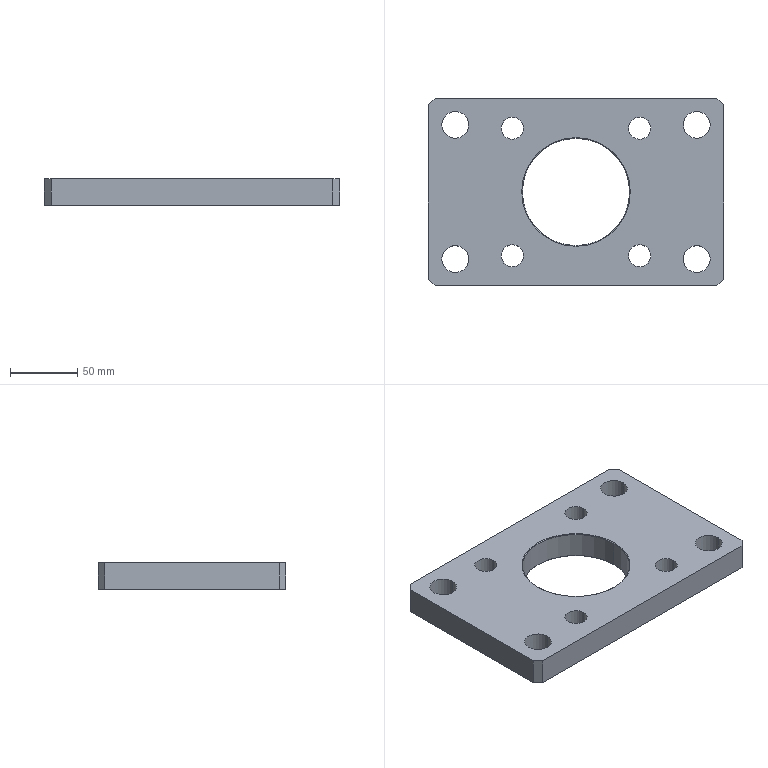Part | SolidWorks | features BaseBody 1 | 1 solid | 32 faces | box 220 x 140 x 20 mm | volume 472167 mm3 | cylinder 18 | plane 10 | cone 4 | commonest cylinder face diameters 16.5 x8 20 x8 80 x2
STEP:
#1=CARTESIAN_POINT('',(-40.,0.,19.5));
#2=VERTEX_POINT('',#1);
#3=CARTESIAN_POINT('',(40.,0.,19.5));
#4=VERTEX_POINT('',#3);
#5=CARTESIAN_POINT('',(0.,0.,19.5));
#6=DIRECTION('',(0.,0.,1.));
#7=DIRECTION('',(1.,0.,0.));
#8=AXIS2_PLACEMENT_3D('',#5,#6,#7);
#9=CIRCLE('',#8,40.);
#10=EDGE_CURVE('',#2,#4,#9,.T.);
#11=ORIENTED_EDGE('',*,*,#10,.F.);
#12=CARTESIAN_POINT('',(-40.5,0.,20.));
#13=VERTEX_POINT('',#12);
#14=CARTESIAN_POINT('',(-40.,0.,19.5));
#15=DIRECTION('',(-0.7071,0.,0.7071));
#16=VECTOR('',#15,1000.);
#17=LINE('',#14,#16);
#18=EDGE_CURVE('',#2,#13,#17,.T.);
#19=ORIENTED_EDGE('',*,*,#18,.T.);
#20=CARTESIAN_POINT('',(40.5,0.,20.));
#21=VERTEX_POINT('',#20);
#22=CARTESIAN_POINT('',(0.,0.,20.));
#23=DIRECTION('',(0.,0.,-1.));
#24=DIRECTION('',(1.,0.,0.));
#25=AXIS2_PLACEMENT_3D('',#22,#23,#24);
#26=CIRCLE('',#25,40.5);
#27=EDGE_CURVE('',#21,#13,#26,.T.);
#28=ORIENTED_EDGE('',*,*,#27,.F.);
#29=CARTESIAN_POINT('',(40.,0.,19.5));
#30=DIRECTION('',(0.7071,0.,0.7071));
#31=VECTOR('',#30,1000.);
#32=LINE('',#29,#31);
#33=EDGE_CURVE('',#4,#21,#32,.T.);
#34=ORIENTED_EDGE('',*,*,#33,.F.);
#35=EDGE_LOOP('',(#11,#19,#28,#34));
#36=FACE_OUTER_BOUND('',#35,.T.);
#37=CARTESIAN_POINT('',(0.,0.,19.5));
#38=DIRECTION('',(0.,0.,1.));
#39=DIRECTION('',(1.,0.,0.));
#40=AXIS2_PLACEMENT_3D('',#37,#38,#39);
#41=CONICAL_SURFACE('',#40,40.,0.7854);
#42=ADVANCED_FACE('',(#36),#41,.F.);
#43=CARTESIAN_POINT('',(40.,0.,0.5));
#44=VERTEX_POINT('',#43);
#45=CARTESIAN_POINT('',(-40.,0.,0.5));
#46=VERTEX_POINT('',#45);
#47=CARTESIAN_POINT('',(0.,0.,0.5));
#48=DIRECTION('',(0.,0.,-1.));
#49=DIRECTION('',(1.,0.,0.));
#50=AXIS2_PLACEMENT_3D('',#47,#48,#49);
#51=CIRCLE('',#50,40.);
#52=EDGE_CURVE('',#44,#46,#51,.T.);
#53=ORIENTED_EDGE('',*,*,#52,.F.);
#54=CARTESIAN_POINT('',(40.5,0.,0.));
#55=VERTEX_POINT('',#54);
#56=CARTESIAN_POINT('',(40.5,0.,0.));
#57=DIRECTION('',(0.7071,0.,-0.7071));
#58=VECTOR('',#57,1000.);
#59=LINE('',#56,#58);
#60=EDGE_CURVE('',#44,#55,#59,.T.);
#61=ORIENTED_EDGE('',*,*,#60,.T.);
#62=CARTESIAN_POINT('',(-40.5,0.,0.));
#63=VERTEX_POINT('',#62);
#64=CARTESIAN_POINT('',(0.,0.,0.));
#65=DIRECTION('',(0.,0.,1.));
#66=DIRECTION('',(1.,0.,0.));
#67=AXIS2_PLACEMENT_3D('',#64,#65,#66);
#68=CIRCLE('',#67,40.5);
#69=EDGE_CURVE('',#63,#55,#68,.T.);
#70=ORIENTED_EDGE('',*,*,#69,.F.);
#71=CARTESIAN_POINT('',(-40.5,0.,0.));
#72=DIRECTION('',(-0.7071,0.,-0.7071));
#73=VECTOR('',#72,1000.);
#74=LINE('',#71,#73);
#75=EDGE_CURVE('',#46,#63,#74,.T.);
#76=ORIENTED_EDGE('',*,*,#75,.F.);
#77=EDGE_LOOP('',(#53,#61,#70,#76));
#78=FACE_OUTER_BOUND('',#77,.T.);
#79=CARTESIAN_POINT('',(0.,0.,0.));
#80=DIRECTION('',(0.,0.,-1.));
#81=DIRECTION('',(-1.,0.,0.));
#82=AXIS2_PLACEMENT_3D('',#79,#80,#81);
#83=CONICAL_SURFACE('',#82,40.5,0.7854);
#84=ADVANCED_FACE('',(#78),#83,.F.);
#85=CARTESIAN_POINT('',(39.25,47.5,0.));
#86=VERTEX_POINT('',#85);
#87=CARTESIAN_POINT('',(55.75,47.5,0.));
#88=VERTEX_POINT('',#87);
#89=CARTESIAN_POINT('',(47.5,47.5,0.));
#90=DIRECTION('',(0.,0.,1.));
#91=DIRECTION('',(1.,0.,0.));
#92=AXIS2_PLACEMENT_3D('',#89,#90,#91);
#93=CIRCLE('',#92,8.25);
#94=EDGE_CURVE('',#86,#88,#93,.T.);
#95=ORIENTED_EDGE('',*,*,#94,.F.);
#96=CARTESIAN_POINT('',(39.25,47.5,20.));
#97=VERTEX_POINT('',#96);
#98=CARTESIAN_POINT('',(39.25,47.5,20.));
#99=DIRECTION('',(0.,0.,1.));
#100=VECTOR('',#99,1000.);
#101=LINE('',#98,#100);
#102=EDGE_CURVE('',#86,#97,#101,.T.);
#103=ORIENTED_EDGE('',*,*,#102,.T.);
#104=CARTESIAN_POINT('',(55.75,47.5,20.));
#105=VERTEX_POINT('',#104);
#106=CARTESIAN_POINT('',(47.5,47.5,20.));
#107=DIRECTION('',(0.,0.,1.));
#108=DIRECTION('',(1.,0.,0.));
#109=AXIS2_PLACEMENT_3D('',#106,#107,#108);
#110=CIRCLE('',#109,8.25);
#111=EDGE_CURVE('',#97,#105,#110,.T.);
#112=ORIENTED_EDGE('',*,*,#111,.T.);
#113=CARTESIAN_POINT('',(55.75,47.5,20.));
#114=DIRECTION('',(0.,0.,1.));
#115=VECTOR('',#114,1000.);
#116=LINE('',#113,#115);
#117=EDGE_CURVE('',#88,#105,#116,.T.);
#118=ORIENTED_EDGE('',*,*,#117,.F.);
#119=EDGE_LOOP('',(#95,#103,#112,#118));
#120=FACE_OUTER_BOUND('',#119,.T.);
#121=CARTESIAN_POINT('',(47.5,47.5,20.));
#122=DIRECTION('',(0.,0.,1.));
#123=DIRECTION('',(1.,0.,0.));
#124=AXIS2_PLACEMENT_3D('',#121,#122,#123);
#125=CYLINDRICAL_SURFACE('',#124,8.25);
#126=ADVANCED_FACE('',(#120),#125,.F.);
#127=CARTESIAN_POINT('',(39.25,-47.5,0.));
#128=VERTEX_POINT('',#127);
#129=CARTESIAN_POINT('',(55.75,-47.5,0.));
#130=VERTEX_POINT('',#129);
#131=CARTESIAN_POINT('',(47.5,-47.5,0.));
#132=DIRECTION('',(0.,0.,1.));
#133=DIRECTION('',(1.,0.,0.));
#134=AXIS2_PLACEMENT_3D('',#131,#132,#133);
#135=CIRCLE('',#134,8.25);
#136=EDGE_CURVE('',#128,#130,#135,.T.);
#137=ORIENTED_EDGE('',*,*,#136,.F.);
#138=CARTESIAN_POINT('',(39.25,-47.5,20.));
#139=VERTEX_POINT('',#138);
#140=CARTESIAN_POINT('',(39.25,-47.5,20.));
#141=DIRECTION('',(0.,0.,1.));
#142=VECTOR('',#141,1000.);
#143=LINE('',#140,#142);
#144=EDGE_CURVE('',#128,#139,#143,.T.);
#145=ORIENTED_EDGE('',*,*,#144,.T.);
#146=CARTESIAN_POINT('',(55.75,-47.5,20.));
#147=VERTEX_POINT('',#146);
#148=CARTESIAN_POINT('',(47.5,-47.5,20.));
#149=DIRECTION('',(0.,0.,1.));
#150=DIRECTION('',(1.,0.,0.));
#151=AXIS2_PLACEMENT_3D('',#148,#149,#150);
#152=CIRCLE('',#151,8.25);
#153=EDGE_CURVE('',#139,#147,#152,.T.);
#154=ORIENTED_EDGE('',*,*,#153,.T.);
#155=CARTESIAN_POINT('',(55.75,-47.5,20.));
#156=DIRECTION('',(0.,0.,1.));
#157=VECTOR('',#156,1000.);
#158=LINE('',#155,#157);
#159=EDGE_CURVE('',#130,#147,#158,.T.);
#160=ORIENTED_EDGE('',*,*,#159,.F.);
#161=EDGE_LOOP('',(#137,#145,#154,#160));
#162=FACE_OUTER_BOUND('',#161,.T.);
#163=CARTESIAN_POINT('',(47.5,-47.5,20.));
#164=DIRECTION('',(0.,0.,1.));
#165=DIRECTION('',(1.,0.,0.));
#166=AXIS2_PLACEMENT_3D('',#163,#164,#165);
#167=CYLINDRICAL_SURFACE('',#166,8.25);
#168=ADVANCED_FACE('',(#162),#167,.F.);
#169=CARTESIAN_POINT('',(-55.75,-47.5,0.));
#170=VERTEX_POINT('',#169);
#171=CARTESIAN_POINT('',(-39.25,-47.5,0.));
#172=VERTEX_POINT('',#171);
#173=CARTESIAN_POINT('',(-47.5,-47.5,0.));
#174=DIRECTION('',(0.,0.,1.));
#175=DIRECTION('',(1.,0.,0.));
#176=AXIS2_PLACEMENT_3D('',#173,#174,#175);
#177=CIRCLE('',#176,8.25);
#178=EDGE_CURVE('',#170,#172,#177,.T.);
#179=ORIENTED_EDGE('',*,*,#178,.F.);
#180=CARTESIAN_POINT('',(-55.75,-47.5,20.));
#181=VERTEX_POINT('',#180);
#182=CARTESIAN_POINT('',(-55.75,-47.5,20.));
#183=DIRECTION('',(0.,0.,1.));
#184=VECTOR('',#183,1000.);
#185=LINE('',#182,#184);
#186=EDGE_CURVE('',#170,#181,#185,.T.);
#187=ORIENTED_EDGE('',*,*,#186,.T.);
#188=CARTESIAN_POINT('',(-39.25,-47.5,20.));
#189=VERTEX_POINT('',#188);
#190=CARTESIAN_POINT('',(-47.5,-47.5,20.));
#191=DIRECTION('',(0.,0.,1.));
#192=DIRECTION('',(1.,0.,0.));
#193=AXIS2_PLACEMENT_3D('',#190,#191,#192);
#194=CIRCLE('',#193,8.25);
#195=EDGE_CURVE('',#181,#189,#194,.T.);
#196=ORIENTED_EDGE('',*,*,#195,.T.);
#197=CARTESIAN_POINT('',(-39.25,-47.5,20.));
#198=DIRECTION('',(0.,0.,1.));
#199=VECTOR('',#198,1000.);
#200=LINE('',#197,#199);
#201=EDGE_CURVE('',#172,#189,#200,.T.);
#202=ORIENTED_EDGE('',*,*,#201,.F.);
#203=EDGE_LOOP('',(#179,#187,#196,#202));
#204=FACE_OUTER_BOUND('',#203,.T.);
#205=CARTESIAN_POINT('',(-47.5,-47.5,20.));
#206=DIRECTION('',(0.,0.,1.));
#207=DIRECTION('',(1.,0.,0.));
#208=AXIS2_PLACEMENT_3D('',#205,#206,#207);
#209=CYLINDRICAL_SURFACE('',#208,8.25);
#210=ADVANCED_FACE('',(#204),#209,.F.);
#211=CARTESIAN_POINT('',(-55.75,47.5,0.));
#212=VERTEX_POINT('',#211);
#213=CARTESIAN_POINT('',(-39.25,47.5,0.));
#214=VERTEX_POINT('',#213);
#215=CARTESIAN_POINT('',(-47.5,47.5,0.));
#216=DIRECTION('',(0.,0.,1.));
#217=DIRECTION('',(1.,0.,0.));
#218=AXIS2_PLACEMENT_3D('',#215,#216,#217);
#219=CIRCLE('',#218,8.25);
#220=EDGE_CURVE('',#212,#214,#219,.T.);
#221=ORIENTED_EDGE('',*,*,#220,.F.);
#222=CARTESIAN_POINT('',(-55.75,47.5,20.));
#223=VERTEX_POINT('',#222);
#224=CARTESIAN_POINT('',(-55.75,47.5,20.));
#225=DIRECTION('',(0.,0.,1.));
#226=VECTOR('',#225,1000.);
#227=LINE('',#224,#226);
#228=EDGE_CURVE('',#212,#223,#227,.T.);
#229=ORIENTED_EDGE('',*,*,#228,.T.);
#230=CARTESIAN_POINT('',(-39.25,47.5,20.));
#231=VERTEX_POINT('',#230);
#232=CARTESIAN_POINT('',(-47.5,47.5,20.));
#233=DIRECTION('',(0.,0.,1.));
#234=DIRECTION('',(1.,0.,0.));
#235=AXIS2_PLACEMENT_3D('',#232,#233,#234);
#236=CIRCLE('',#235,8.25);
#237=EDGE_CURVE('',#223,#231,#236,.T.);
#238=ORIENTED_EDGE('',*,*,#237,.T.);
#239=CARTESIAN_POINT('',(-39.25,47.5,20.));
#240=DIRECTION('',(0.,0.,1.));
#241=VECTOR('',#240,1000.);
#242=LINE('',#239,#241);
#243=EDGE_CURVE('',#214,#231,#242,.T.);
#244=ORIENTED_EDGE('',*,*,#243,.F.);
#245=EDGE_LOOP('',(#221,#229,#238,#244));
#246=FACE_OUTER_BOUND('',#245,.T.);
#247=CARTESIAN_POINT('',(-47.5,47.5,20.));
#248=DIRECTION('',(0.,0.,1.));
#249=DIRECTION('',(1.,0.,0.));
#250=AXIS2_PLACEMENT_3D('',#247,#248,#249);
#251=CYLINDRICAL_SURFACE('',#250,8.25);
#252=ADVANCED_FACE('',(#246),#251,.F.);
#253=CARTESIAN_POINT('',(-100.,50.,0.));
#254=VERTEX_POINT('',#253);
#255=CARTESIAN_POINT('',(-80.,50.,0.));
#256=VERTEX_POINT('',#255);
#257=CARTESIAN_POINT('',(-90.,50.,0.));
#258=DIRECTION('',(0.,0.,1.));
#259=DIRECTION('',(1.,0.,0.));
#260=AXIS2_PLACEMENT_3D('',#257,#258,#259);
#261=CIRCLE('',#260,10.);
#262=EDGE_CURVE('',#254,#256,#261,.T.);
#263=ORIENTED_EDGE('',*,*,#262,.F.);
#264=CARTESIAN_POINT('',(-100.,50.,20.));
#265=VERTEX_POINT('',#264);
#266=CARTESIAN_POINT('',(-100.,50.,20.));
#267=DIRECTION('',(0.,0.,1.));
#268=VECTOR('',#267,1000.);
#269=LINE('',#266,#268);
#270=EDGE_CURVE('',#254,#265,#269,.T.);
#271=ORIENTED_EDGE('',*,*,#270,.T.);
#272=CARTESIAN_POINT('',(-80.,50.,20.));
#273=VERTEX_POINT('',#272);
#274=CARTESIAN_POINT('',(-90.,50.,20.));
#275=DIRECTION('',(0.,0.,1.));
#276=DIRECTION('',(1.,0.,0.));
#277=AXIS2_PLACEMENT_3D('',#274,#275,#276);
#278=CIRCLE('',#277,10.);
#279=EDGE_CURVE('',#265,#273,#278,.T.);
#280=ORIENTED_EDGE('',*,*,#279,.T.);
#281=CARTESIAN_POINT('',(-80.,50.,20.));
#282=DIRECTION('',(0.,0.,1.));
#283=VECTOR('',#282,1000.);
#284=LINE('',#281,#283);
#285=EDGE_CURVE('',#256,#273,#284,.T.);
#286=ORIENTED_EDGE('',*,*,#285,.F.);
#287=EDGE_LOOP('',(#263,#271,#280,#286));
#288=FACE_OUTER_BOUND('',#287,.T.);
#289=CARTESIAN_POINT('',(-90.,50.,20.));
#290=DIRECTION('',(0.,0.,1.));
#291=DIRECTION('',(1.,0.,0.));
#292=AXIS2_PLACEMENT_3D('',#289,#290,#291);
#293=CYLINDRICAL_SURFACE('',#292,10.);
#294=ADVANCED_FACE('',(#288),#293,.F.);
#295=CARTESIAN_POINT('',(-100.,-50.,0.));
#296=VERTEX_POINT('',#295);
#297=CARTESIAN_POINT('',(-80.,-50.,0.));
#298=VERTEX_POINT('',#297);
#299=CARTESIAN_POINT('',(-90.,-50.,0.));
#300=DIRECTION('',(0.,0.,1.));
#301=DIRECTION('',(1.,0.,0.));
#302=AXIS2_PLACEMENT_3D('',#299,#300,#301);
#303=CIRCLE('',#302,10.);
#304=EDGE_CURVE('',#296,#298,#303,.T.);
#305=ORIENTED_EDGE('',*,*,#304,.F.);
#306=CARTESIAN_POINT('',(-100.,-50.,20.));
#307=VERTEX_POINT('',#306);
#308=CARTESIAN_POINT('',(-100.,-50.,20.));
#309=DIRECTION('',(0.,0.,1.));
#310=VECTOR('',#309,1000.);
#311=LINE('',#308,#310);
#312=EDGE_CURVE('',#296,#307,#311,.T.);
#313=ORIENTED_EDGE('',*,*,#312,.T.);
#314=CARTESIAN_POINT('',(-80.,-50.,20.));
#315=VERTEX_POINT('',#314);
#316=CARTESIAN_POINT('',(-90.,-50.,20.));
#317=DIRECTION('',(0.,0.,1.));
#318=DIRECTION('',(1.,0.,0.));
#319=AXIS2_PLACEMENT_3D('',#316,#317,#318);
#320=CIRCLE('',#319,10.);
#321=EDGE_CURVE('',#307,#315,#320,.T.);
#322=ORIENTED_EDGE('',*,*,#321,.T.);
#323=CARTESIAN_POINT('',(-80.,-50.,20.));
#324=DIRECTION('',(0.,0.,1.));
#325=VECTOR('',#324,1000.);
#326=LINE('',#323,#325);
#327=EDGE_CURVE('',#298,#315,#326,.T.);
#328=ORIENTED_EDGE('',*,*,#327,.F.);
#329=EDGE_LOOP('',(#305,#313,#322,#328));
#330=FACE_OUTER_BOUND('',#329,.T.);
#331=CARTESIAN_POINT('',(-90.,-50.,20.));
#332=DIRECTION('',(0.,0.,1.));
#333=DIRECTION('',(1.,0.,0.));
#334=AXIS2_PLACEMENT_3D('',#331,#332,#333);
#335=CYLINDRICAL_SURFACE('',#334,10.);
#336=ADVANCED_FACE('',(#330),#335,.F.);
#337=CARTESIAN_POINT('',(80.,50.,0.));
#338=VERTEX_POINT('',#337);
#339=CARTESIAN_POINT('',(100.,50.,0.));
#340=VERTEX_POINT('',#339);
#341=CARTESIAN_POINT('',(90.,50.,0.));
#342=DIRECTION('',(0.,0.,1.));
#343=DIRECTION('',(1.,0.,0.));
#344=AXIS2_PLACEMENT_3D('',#341,#342,#343);
#345=CIRCLE('',#344,10.);
#346=EDGE_CURVE('',#338,#340,#345,.T.);
#347=ORIENTED_EDGE('',*,*,#346,.F.);
#348=CARTESIAN_POINT('',(80.,50.,20.));
#349=VERTEX_POINT('',#348);
#350=CARTESIAN_POINT('',(80.,50.,20.));
#351=DIRECTION('',(0.,0.,1.));
#352=VECTOR('',#351,1000.);
#353=LINE('',#350,#352);
#354=EDGE_CURVE('',#338,#349,#353,.T.);
#355=ORIENTED_EDGE('',*,*,#354,.T.);
#356=CARTESIAN_POINT('',(100.,50.,20.));
#357=VERTEX_POINT('',#356);
#358=CARTESIAN_POINT('',(90.,50.,20.));
#359=DIRECTION('',(0.,0.,1.));
#360=DIRECTION('',(1.,0.,0.));
#361=AXIS2_PLACEMENT_3D('',#358,#359,#360);
#362=CIRCLE('',#361,10.);
#363=EDGE_CURVE('',#349,#357,#362,.T.);
#364=ORIENTED_EDGE('',*,*,#363,.T.);
#365=CARTESIAN_POINT('',(100.,50.,20.));
#366=DIRECTION('',(0.,0.,1.));
#367=VECTOR('',#366,1000.);
#368=LINE('',#365,#367);
#369=EDGE_CURVE('',#340,#357,#368,.T.);
#370=ORIENTED_EDGE('',*,*,#369,.F.);
#371=EDGE_LOOP('',(#347,#355,#364,#370));
#372=FACE_OUTER_BOUND('',#371,.T.);
#373=CARTESIAN_POINT('',(90.,50.,20.));
#374=DIRECTION('',(0.,0.,1.));
#375=DIRECTION('',(1.,0.,0.));
#376=AXIS2_PLACEMENT_3D('',#373,#374,#375);
#377=CYLINDRICAL_SURFACE('',#376,10.);
#378=ADVANCED_FACE('',(#372),#377,.F.);
#379=CARTESIAN_POINT('',(80.,-50.,0.));
#380=VERTEX_POINT('',#379);
#381=CARTESIAN_POINT('',(100.,-50.,0.));
#382=VERTEX_POINT('',#381);
#383=CARTESIAN_POINT('',(90.,-50.,0.));
#384=DIRECTION('',(0.,0.,1.));
#385=DIRECTION('',(1.,0.,0.));
#386=AXIS2_PLACEMENT_3D('',#383,#384,#385);
#387=CIRCLE('',#386,10.);
#388=EDGE_CURVE('',#380,#382,#387,.T.);
#389=ORIENTED_EDGE('',*,*,#388,.F.);
#390=CARTESIAN_POINT('',(80.,-50.,20.));
#391=VERTEX_POINT('',#390);
#392=CARTESIAN_POINT('',(80.,-50.,20.));
#393=DIRECTION('',(0.,0.,1.));
#394=VECTOR('',#393,1000.);
#395=LINE('',#392,#394);
#396=EDGE_CURVE('',#380,#391,#395,.T.);
#397=ORIENTED_EDGE('',*,*,#396,.T.);
#398=CARTESIAN_POINT('',(100.,-50.,20.));
#399=VERTEX_POINT('',#398);
#400=CARTESIAN_POINT('',(90.,-50.,20.));
#401=DIRECTION('',(0.,0.,1.));
#402=DIRECTION('',(1.,0.,0.));
#403=AXIS2_PLACEMENT_3D('',#400,#401,#402);
#404=CIRCLE('',#403,10.);
#405=EDGE_CURVE('',#391,#399,#404,.T.);
#406=ORIENTED_EDGE('',*,*,#405,.T.);
#407=CARTESIAN_POINT('',(100.,-50.,20.));
#408=DIRECTION('',(0.,0.,1.));
#409=VECTOR('',#408,1000.);
#410=LINE('',#407,#409);
#411=EDGE_CURVE('',#382,#399,#410,.T.);
#412=ORIENTED_EDGE('',*,*,#411,.F.);
#413=EDGE_LOOP('',(#389,#397,#406,#412));
#414=FACE_OUTER_BOUND('',#413,.T.);
#415=CARTESIAN_POINT('',(90.,-50.,20.));
#416=DIRECTION('',(0.,0.,1.));
#417=DIRECTION('',(1.,0.,0.));
#418=AXIS2_PLACEMENT_3D('',#415,#416,#417);
#419=CYLINDRICAL_SURFACE('',#418,10.);
#420=ADVANCED_FACE('',(#414),#419,.F.);
#421=ORIENTED_EDGE('',*,*,#10,.T.);
#422=CARTESIAN_POINT('',(40.,0.,20.));
#423=DIRECTION('',(0.,0.,-1.));
#424=VECTOR('',#423,1000.);
#425=LINE('',#422,#424);
#426=EDGE_CURVE('',#4,#44,#425,.T.);
#427=ORIENTED_EDGE('',*,*,#426,.T.);
#428=ORIENTED_EDGE('',*,*,#52,.T.);
#429=CARTESIAN_POINT('',(-40.,0.,20.));
#430=DIRECTION('',(0.,0.,-1.));
#431=VECTOR('',#430,1000.);
#432=LINE('',#429,#431);
#433=EDGE_CURVE('',#2,#46,#432,.T.);
#434=ORIENTED_EDGE('',*,*,#433,.F.);
#435=EDGE_LOOP('',(#421,#427,#428,#434));
#436=FACE_OUTER_BOUND('',#435,.T.);
#437=CARTESIAN_POINT('',(0.,0.,20.));
#438=DIRECTION('',(0.,0.,-1.));
#439=DIRECTION('',(-1.,0.,0.));
#440=AXIS2_PLACEMENT_3D('',#437,#438,#439);
#441=CYLINDRICAL_SURFACE('',#440,40.);
#442=ADVANCED_FACE('',(#436),#441,.F.);
#443=CARTESIAN_POINT('',(110.,65.,20.));
#444=VERTEX_POINT('',#443);
#445=CARTESIAN_POINT('',(105.,70.,20.));
#446=VERTEX_POINT('',#445);
#447=CARTESIAN_POINT('',(87.5,87.5,20.));
#448=DIRECTION('',(-0.7071,0.7071,0.));
#449=VECTOR('',#448,1000.);
#450=LINE('',#447,#449);
#451=EDGE_CURVE('',#444,#446,#450,.T.);
#452=ORIENTED_EDGE('',*,*,#451,.F.);
#453=CARTESIAN_POINT('',(110.,65.,0.));
#454=VERTEX_POINT('',#453);
#455=CARTESIAN_POINT('',(110.,65.,20.));
#456=DIRECTION('',(0.,0.,1.));
#457=VECTOR('',#456,1000.);
#458=LINE('',#455,#457);
#459=EDGE_CURVE('',#454,#444,#458,.T.);
#460=ORIENTED_EDGE('',*,*,#459,.F.);
#461=CARTESIAN_POINT('',(105.,70.,0.));
#462=VERTEX_POINT('',#461);
#463=CARTESIAN_POINT('',(105.,70.,0.));
#464=DIRECTION('',(0.7071,-0.7071,0.));
#465=VECTOR('',#464,1000.);
#466=LINE('',#463,#465);
#467=EDGE_CURVE('',#462,#454,#466,.T.);
#468=ORIENTED_EDGE('',*,*,#467,.F.);
#469=CARTESIAN_POINT('',(105.,70.,20.));
#470=DIRECTION('',(0.,0.,-1.));
#471=VECTOR('',#470,1000.);
#472=LINE('',#469,#471);
#473=EDGE_CURVE('',#446,#462,#472,.T.);
#474=ORIENTED_EDGE('',*,*,#473,.F.);
#475=EDGE_LOOP('',(#452,#460,#468,#474));
#476=FACE_OUTER_BOUND('',#475,.T.);
#477=CARTESIAN_POINT('',(105.,70.,20.));
#478=DIRECTION('',(-0.7071,-0.7071,0.));
#479=DIRECTION('',(-0.7071,0.7071,0.));
#480=AXIS2_PLACEMENT_3D('',#477,#478,#479);
#481=PLANE('',#480);
#482=ADVANCED_FACE('',(#476),#481,.F.);
#483=CARTESIAN_POINT('',(105.,-70.,20.));
#484=VERTEX_POINT('',#483);
#485=CARTESIAN_POINT('',(110.,-65.,20.));
#486=VERTEX_POINT('',#485);
#487=CARTESIAN_POINT('',(87.5,-87.5,20.));
#488=DIRECTION('',(0.7071,0.7071,0.));
#489=VECTOR('',#488,1000.);
#490=LINE('',#487,#489);
#491=EDGE_CURVE('',#484,#486,#490,.T.);
#492=ORIENTED_EDGE('',*,*,#491,.F.);
#493=CARTESIAN_POINT('',(105.,-70.,0.));
#494=VERTEX_POINT('',#493);
#495=CARTESIAN_POINT('',(105.,-70.,20.));
#496=DIRECTION('',(0.,0.,1.));
#497=VECTOR('',#496,1000.);
#498=LINE('',#495,#497);
#499=EDGE_CURVE('',#494,#484,#498,.T.);
#500=ORIENTED_EDGE('',*,*,#499,.F.);
#501=CARTESIAN_POINT('',(110.,-65.,0.));
#502=VERTEX_POINT('',#501);
#503=CARTESIAN_POINT('',(110.,-65.,0.));
#504=DIRECTION('',(-0.7071,-0.7071,0.));
#505=VECTOR('',#504,1000.);
#506=LINE('',#503,#505);
#507=EDGE_CURVE('',#502,#494,#506,.T.);
#508=ORIENTED_EDGE('',*,*,#507,.F.);
#509=CARTESIAN_POINT('',(110.,-65.,20.));
#510=DIRECTION('',(0.,0.,-1.));
#511=VECTOR('',#510,1000.);
#512=LINE('',#509,#511);
#513=EDGE_CURVE('',#486,#502,#512,.T.);
#514=ORIENTED_EDGE('',*,*,#513,.F.);
#515=EDGE_LOOP('',(#492,#500,#508,#514));
#516=FACE_OUTER_BOUND('',#515,.T.);
#517=CARTESIAN_POINT('',(110.,-65.,20.));
#518=DIRECTION('',(-0.7071,0.7071,0.));
#519=DIRECTION('',(0.,0.,1.));
#520=AXIS2_PLACEMENT_3D('',#517,#518,#519);
#521=PLANE('',#520);
#522=ADVANCED_FACE('',(#516),#521,.F.);
#523=CARTESIAN_POINT('',(-105.,70.,20.));
#524=VERTEX_POINT('',#523);
#525=CARTESIAN_POINT('',(-110.,65.,20.));
#526=VERTEX_POINT('',#525);
#527=CARTESIAN_POINT('',(-87.5,87.5,20.));
#528=DIRECTION('',(-0.7071,-0.7071,0.));
#529=VECTOR('',#528,1000.);
#530=LINE('',#527,#529);
#531=EDGE_CURVE('',#524,#526,#530,.T.);
#532=ORIENTED_EDGE('',*,*,#531,.F.);
#533=CARTESIAN_POINT('',(-105.,70.,0.));
#534=VERTEX_POINT('',#533);
#535=CARTESIAN_POINT('',(-105.,70.,20.));
#536=DIRECTION('',(0.,0.,1.));
#537=VECTOR('',#536,1000.);
#538=LINE('',#535,#537);
#539=EDGE_CURVE('',#534,#524,#538,.T.);
#540=ORIENTED_EDGE('',*,*,#539,.F.);
#541=CARTESIAN_POINT('',(-110.,65.,0.));
#542=VERTEX_POINT('',#541);
#543=CARTESIAN_POINT('',(-110.,65.,0.));
#544=DIRECTION('',(0.7071,0.7071,0.));
#545=VECTOR('',#544,1000.);
#546=LINE('',#543,#545);
#547=EDGE_CURVE('',#542,#534,#546,.T.);
#548=ORIENTED_EDGE('',*,*,#547,.F.);
#549=CARTESIAN_POINT('',(-110.,65.,20.));
#550=DIRECTION('',(0.,0.,-1.));
#551=VECTOR('',#550,1000.);
#552=LINE('',#549,#551);
#553=EDGE_CURVE('',#526,#542,#552,.T.);
#554=ORIENTED_EDGE('',*,*,#553,.F.);
#555=EDGE_LOOP('',(#532,#540,#548,#554));
#556=FACE_OUTER_BOUND('',#555,.T.);
#557=CARTESIAN_POINT('',(-110.,65.,20.));
#558=DIRECTION('',(0.7071,-0.7071,0.));
#559=DIRECTION('',(0.,0.,-1.));
#560=AXIS2_PLACEMENT_3D('',#557,#558,#559);
#561=PLANE('',#560);
#562=ADVANCED_FACE('',(#556),#561,.F.);
#563=CARTESIAN_POINT('',(-110.,-65.,20.));
#564=VERTEX_POINT('',#563);
#565=CARTESIAN_POINT('',(-105.,-70.,20.));
#566=VERTEX_POINT('',#565);
#567=CARTESIAN_POINT('',(-87.5,-87.5,20.));
#568=DIRECTION('',(0.7071,-0.7071,0.));
#569=VECTOR('',#568,1000.);
#570=LINE('',#567,#569);
#571=EDGE_CURVE('',#564,#566,#570,.T.);
#572=ORIENTED_EDGE('',*,*,#571,.F.);
#573=CARTESIAN_POINT('',(-110.,-65.,0.));
#574=VERTEX_POINT('',#573);
#575=CARTESIAN_POINT('',(-110.,-65.,20.));
#576=DIRECTION('',(0.,0.,1.));
#577=VECTOR('',#576,1000.);
#578=LINE('',#575,#577);
#579=EDGE_CURVE('',#574,#564,#578,.T.);
#580=ORIENTED_EDGE('',*,*,#579,.F.);
#581=CARTESIAN_POINT('',(-105.,-70.,0.));
#582=VERTEX_POINT('',#581);
#583=CARTESIAN_POINT('',(-105.,-70.,0.));
#584=DIRECTION('',(-0.7071,0.7071,0.));
#585=VECTOR('',#584,1000.);
#586=LINE('',#583,#585);
#587=EDGE_CURVE('',#582,#574,#586,.T.);
#588=ORIENTED_EDGE('',*,*,#587,.F.);
#589=CARTESIAN_POINT('',(-105.,-70.,20.));
#590=DIRECTION('',(0.,0.,-1.));
#591=VECTOR('',#590,1000.);
#592=LINE('',#589,#591);
#593=EDGE_CURVE('',#566,#582,#592,.T.);
#594=ORIENTED_EDGE('',*,*,#593,.F.);
#595=EDGE_LOOP('',(#572,#580,#588,#594));
#596=FACE_OUTER_BOUND('',#595,.T.);
#597=CARTESIAN_POINT('',(-105.,-70.,20.));
#598=DIRECTION('',(0.7071,0.7071,0.));
#599=DIRECTION('',(0.,0.,-1.));
#600=AXIS2_PLACEMENT_3D('',#597,#598,#599);
#601=PLANE('',#600);
#602=ADVANCED_FACE('',(#596),#601,.F.);
#603=CARTESIAN_POINT('',(-110.,70.,0.));
#604=DIRECTION('',(-1.,0.,0.));
#605=VECTOR('',#604,1000.);
#606=LINE('',#603,#605);
#607=EDGE_CURVE('',#462,#534,#606,.T.);
#608=ORIENTED_EDGE('',*,*,#607,.T.);
#609=ORIENTED_EDGE('',*,*,#539,.T.);
#610=CARTESIAN_POINT('',(-110.,70.,20.));
#611=DIRECTION('',(-1.,0.,0.));
#612=VECTOR('',#611,1000.);
#613=LINE('',#610,#612);
#614=EDGE_CURVE('',#446,#524,#613,.T.);
#615=ORIENTED_EDGE('',*,*,#614,.F.);
#616=ORIENTED_EDGE('',*,*,#473,.T.);
#617=EDGE_LOOP('',(#608,#609,#615,#616));
#618=FACE_OUTER_BOUND('',#617,.T.);
#619=CARTESIAN_POINT('',(-110.,70.,20.));
#620=DIRECTION('',(0.,-1.,0.));
#621=DIRECTION('',(0.,0.,-1.));
#622=AXIS2_PLACEMENT_3D('',#619,#620,#621);
#623=PLANE('',#622);
#624=ADVANCED_FACE('',(#618),#623,.F.);
#625=CARTESIAN_POINT('',(110.,70.,20.));
#626=DIRECTION('',(0.,1.,0.));
#627=VECTOR('',#626,1000.);
#628=LINE('',#625,#627);
#629=EDGE_CURVE('',#486,#444,#628,.T.);
#630=ORIENTED_EDGE('',*,*,#629,.F.);
#631=ORIENTED_EDGE('',*,*,#513,.T.);
#632=CARTESIAN_POINT('',(110.,70.,0.));
#633=DIRECTION('',(0.,1.,0.));
#634=VECTOR('',#633,1000.);
#635=LINE('',#632,#634);
#636=EDGE_CURVE('',#502,#454,#635,.T.);
#637=ORIENTED_EDGE('',*,*,#636,.T.);
#638=ORIENTED_EDGE('',*,*,#459,.T.);
#639=EDGE_LOOP('',(#630,#631,#637,#638));
#640=FACE_OUTER_BOUND('',#639,.T.);
#641=CARTESIAN_POINT('',(110.,70.,20.));
#642=DIRECTION('',(-1.,0.,0.));
#643=DIRECTION('',(0.,1.,0.));
#644=AXIS2_PLACEMENT_3D('',#641,#642,#643);
#645=PLANE('',#644);
#646=ADVANCED_FACE('',(#640),#645,.F.);
#647=CARTESIAN_POINT('',(-110.,-70.,20.));
#648=DIRECTION('',(1.,0.,0.));
#649=VECTOR('',#648,1000.);
#650=LINE('',#647,#649);
#651=EDGE_CURVE('',#566,#484,#650,.T.);
#652=ORIENTED_EDGE('',*,*,#651,.F.);
#653=ORIENTED_EDGE('',*,*,#593,.T.);
#654=CARTESIAN_POINT('',(-110.,-70.,0.));
#655=DIRECTION('',(1.,0.,0.));
#656=VECTOR('',#655,1000.);
#657=LINE('',#654,#656);
#658=EDGE_CURVE('',#582,#494,#657,.T.);
#659=ORIENTED_EDGE('',*,*,#658,.T.);
#660=ORIENTED_EDGE('',*,*,#499,.T.);
#661=EDGE_LOOP('',(#652,#653,#659,#660));
#662=FACE_OUTER_BOUND('',#661,.T.);
#663=CARTESIAN_POINT('',(-110.,-70.,20.));
#664=DIRECTION('',(0.,1.,0.));
#665=DIRECTION('',(1.,0.,0.));
#666=AXIS2_PLACEMENT_3D('',#663,#664,#665);
#667=PLANE('',#666);
#668=ADVANCED_FACE('',(#662),#667,.F.);
#669=CARTESIAN_POINT('',(-110.,70.,0.));
#670=DIRECTION('',(0.,-1.,0.));
#671=VECTOR('',#670,1000.);
#672=LINE('',#669,#671);
#673=EDGE_CURVE('',#542,#574,#672,.T.);
#674=ORIENTED_EDGE('',*,*,#673,.T.);
#675=ORIENTED_EDGE('',*,*,#579,.T.);
#676=CARTESIAN_POINT('',(-110.,70.,20.));
#677=DIRECTION('',(0.,-1.,0.));
#678=VECTOR('',#677,1000.);
#679=LINE('',#676,#678);
#680=EDGE_CURVE('',#526,#564,#679,.T.);
#681=ORIENTED_EDGE('',*,*,#680,.F.);
#682=ORIENTED_EDGE('',*,*,#553,.T.);
#683=EDGE_LOOP('',(#674,#675,#681,#682));
#684=FACE_OUTER_BOUND('',#683,.T.);
#685=CARTESIAN_POINT('',(-110.,70.,20.));
#686=DIRECTION('',(1.,0.,0.));
#687=DIRECTION('',(0.,1.,0.));
#688=AXIS2_PLACEMENT_3D('',#685,#686,#687);
#689=PLANE('',#688);
#690=ADVANCED_FACE('',(#684),#689,.F.);
#691=CARTESIAN_POINT('',(90.,-50.,0.));
#692=DIRECTION('',(0.,0.,1.));
#693=DIRECTION('',(1.,0.,0.));
#694=AXIS2_PLACEMENT_3D('',#691,#692,#693);
#695=CIRCLE('',#694,10.);
#696=EDGE_CURVE('',#382,#380,#695,.T.);
#697=ORIENTED_EDGE('',*,*,#696,.T.);
#698=ORIENTED_EDGE('',*,*,#388,.T.);
#699=EDGE_LOOP('',(#697,#698));
#700=FACE_BOUND('',#699,.T.);
#701=CARTESIAN_POINT('',(90.,50.,0.));
#702=DIRECTION('',(0.,0.,1.));
#703=DIRECTION('',(1.,0.,0.));
#704=AXIS2_PLACEMENT_3D('',#701,#702,#703);
#705=CIRCLE('',#704,10.);
#706=EDGE_CURVE('',#340,#338,#705,.T.);
#707=ORIENTED_EDGE('',*,*,#706,.T.);
#708=ORIENTED_EDGE('',*,*,#346,.T.);
#709=EDGE_LOOP('',(#707,#708));
#710=FACE_BOUND('',#709,.T.);
#711=CARTESIAN_POINT('',(-90.,-50.,0.));
#712=DIRECTION('',(0.,0.,1.));
#713=DIRECTION('',(1.,0.,0.));
#714=AXIS2_PLACEMENT_3D('',#711,#712,#713);
#715=CIRCLE('',#714,10.);
#716=EDGE_CURVE('',#298,#296,#715,.T.);
#717=ORIENTED_EDGE('',*,*,#716,.T.);
#718=ORIENTED_EDGE('',*,*,#304,.T.);
#719=EDGE_LOOP('',(#717,#718));
#720=FACE_BOUND('',#719,.T.);
#721=CARTESIAN_POINT('',(-90.,50.,0.));
#722=DIRECTION('',(0.,0.,1.));
#723=DIRECTION('',(1.,0.,0.));
#724=AXIS2_PLACEMENT_3D('',#721,#722,#723);
#725=CIRCLE('',#724,10.);
#726=EDGE_CURVE('',#256,#254,#725,.T.);
#727=ORIENTED_EDGE('',*,*,#726,.T.);
#728=ORIENTED_EDGE('',*,*,#262,.T.);
#729=EDGE_LOOP('',(#727,#728));
#730=FACE_BOUND('',#729,.T.);
#731=CARTESIAN_POINT('',(-47.5,47.5,0.));
#732=DIRECTION('',(0.,0.,1.));
#733=DIRECTION('',(1.,0.,0.));
#734=AXIS2_PLACEMENT_3D('',#731,#732,#733);
#735=CIRCLE('',#734,8.25);
#736=EDGE_CURVE('',#214,#212,#735,.T.);
#737=ORIENTED_EDGE('',*,*,#736,.T.);
#738=ORIENTED_EDGE('',*,*,#220,.T.);
#739=EDGE_LOOP('',(#737,#738));
#740=FACE_BOUND('',#739,.T.);
#741=CARTESIAN_POINT('',(-47.5,-47.5,0.));
#742=DIRECTION('',(0.,0.,1.));
#743=DIRECTION('',(1.,0.,0.));
#744=AXIS2_PLACEMENT_3D('',#741,#742,#743);
#745=CIRCLE('',#744,8.25);
#746=EDGE_CURVE('',#172,#170,#745,.T.);
#747=ORIENTED_EDGE('',*,*,#746,.T.);
#748=ORIENTED_EDGE('',*,*,#178,.T.);
#749=EDGE_LOOP('',(#747,#748));
#750=FACE_BOUND('',#749,.T.);
#751=CARTESIAN_POINT('',(47.5,-47.5,0.));
#752=DIRECTION('',(0.,0.,1.));
#753=DIRECTION('',(1.,0.,0.));
#754=AXIS2_PLACEMENT_3D('',#751,#752,#753);
#755=CIRCLE('',#754,8.25);
#756=EDGE_CURVE('',#130,#128,#755,.T.);
#757=ORIENTED_EDGE('',*,*,#756,.T.);
#758=ORIENTED_EDGE('',*,*,#136,.T.);
#759=EDGE_LOOP('',(#757,#758));
#760=FACE_BOUND('',#759,.T.);
#761=CARTESIAN_POINT('',(47.5,47.5,0.));
#762=DIRECTION('',(0.,0.,1.));
#763=DIRECTION('',(1.,0.,0.));
#764=AXIS2_PLACEMENT_3D('',#761,#762,#763);
#765=CIRCLE('',#764,8.25);
#766=EDGE_CURVE('',#88,#86,#765,.T.);
#767=ORIENTED_EDGE('',*,*,#766,.T.);
#768=ORIENTED_EDGE('',*,*,#94,.T.);
#769=EDGE_LOOP('',(#767,#768));
#770=FACE_BOUND('',#769,.T.);
#771=ORIENTED_EDGE('',*,*,#69,.T.);
#772=CARTESIAN_POINT('',(0.,0.,0.));
#773=DIRECTION('',(0.,0.,1.));
#774=DIRECTION('',(1.,0.,0.));
#775=AXIS2_PLACEMENT_3D('',#772,#773,#774);
#776=CIRCLE('',#775,40.5);
#777=EDGE_CURVE('',#55,#63,#776,.T.);
#778=ORIENTED_EDGE('',*,*,#777,.T.);
#779=EDGE_LOOP('',(#771,#778));
#780=FACE_BOUND('',#779,.T.);
#781=ORIENTED_EDGE('',*,*,#658,.F.);
#782=ORIENTED_EDGE('',*,*,#587,.T.);
#783=ORIENTED_EDGE('',*,*,#673,.F.);
#784=ORIENTED_EDGE('',*,*,#547,.T.);
#785=ORIENTED_EDGE('',*,*,#607,.F.);
#786=ORIENTED_EDGE('',*,*,#467,.T.);
#787=ORIENTED_EDGE('',*,*,#636,.F.);
#788=ORIENTED_EDGE('',*,*,#507,.T.);
#789=EDGE_LOOP('',(#781,#782,#783,#784,#785,#786,#787,#788));
#790=FACE_OUTER_BOUND('',#789,.T.);
#791=CARTESIAN_POINT('',(0.,0.,0.));
#792=DIRECTION('',(0.,0.,1.));
#793=DIRECTION('',(1.,0.,0.));
#794=AXIS2_PLACEMENT_3D('',#791,#792,#793);
#795=PLANE('',#794);
#796=ADVANCED_FACE('',(#700,#710,#720,#730,#740,#750,#760,#770,#780,#790),#795,.F.);
#797=CARTESIAN_POINT('',(90.,-50.,20.));
#798=DIRECTION('',(0.,0.,1.));
#799=DIRECTION('',(1.,0.,0.));
#800=AXIS2_PLACEMENT_3D('',#797,#798,#799);
#801=CIRCLE('',#800,10.);
#802=EDGE_CURVE('',#399,#391,#801,.T.);
#803=ORIENTED_EDGE('',*,*,#802,.F.);
#804=ORIENTED_EDGE('',*,*,#405,.F.);
#805=EDGE_LOOP('',(#803,#804));
#806=FACE_BOUND('',#805,.T.);
#807=CARTESIAN_POINT('',(90.,50.,20.));
#808=DIRECTION('',(0.,0.,1.));
#809=DIRECTION('',(1.,0.,0.));
#810=AXIS2_PLACEMENT_3D('',#807,#808,#809);
#811=CIRCLE('',#810,10.);
#812=EDGE_CURVE('',#357,#349,#811,.T.);
#813=ORIENTED_EDGE('',*,*,#812,.F.);
#814=ORIENTED_EDGE('',*,*,#363,.F.);
#815=EDGE_LOOP('',(#813,#814));
#816=FACE_BOUND('',#815,.T.);
#817=CARTESIAN_POINT('',(-90.,-50.,20.));
#818=DIRECTION('',(0.,0.,1.));
#819=DIRECTION('',(1.,0.,0.));
#820=AXIS2_PLACEMENT_3D('',#817,#818,#819);
#821=CIRCLE('',#820,10.);
#822=EDGE_CURVE('',#315,#307,#821,.T.);
#823=ORIENTED_EDGE('',*,*,#822,.F.);
#824=ORIENTED_EDGE('',*,*,#321,.F.);
#825=EDGE_LOOP('',(#823,#824));
#826=FACE_BOUND('',#825,.T.);
#827=CARTESIAN_POINT('',(-90.,50.,20.));
#828=DIRECTION('',(0.,0.,1.));
#829=DIRECTION('',(1.,0.,0.));
#830=AXIS2_PLACEMENT_3D('',#827,#828,#829);
#831=CIRCLE('',#830,10.);
#832=EDGE_CURVE('',#273,#265,#831,.T.);
#833=ORIENTED_EDGE('',*,*,#832,.F.);
#834=ORIENTED_EDGE('',*,*,#279,.F.);
#835=EDGE_LOOP('',(#833,#834));
#836=FACE_BOUND('',#835,.T.);
#837=CARTESIAN_POINT('',(-47.5,47.5,20.));
#838=DIRECTION('',(0.,0.,1.));
#839=DIRECTION('',(1.,0.,0.));
#840=AXIS2_PLACEMENT_3D('',#837,#838,#839);
#841=CIRCLE('',#840,8.25);
#842=EDGE_CURVE('',#231,#223,#841,.T.);
#843=ORIENTED_EDGE('',*,*,#842,.F.);
#844=ORIENTED_EDGE('',*,*,#237,.F.);
#845=EDGE_LOOP('',(#843,#844));
#846=FACE_BOUND('',#845,.T.);
#847=CARTESIAN_POINT('',(-47.5,-47.5,20.));
#848=DIRECTION('',(0.,0.,1.));
#849=DIRECTION('',(1.,0.,0.));
#850=AXIS2_PLACEMENT_3D('',#847,#848,#849);
#851=CIRCLE('',#850,8.25);
#852=EDGE_CURVE('',#189,#181,#851,.T.);
#853=ORIENTED_EDGE('',*,*,#852,.F.);
#854=ORIENTED_EDGE('',*,*,#195,.F.);
#855=EDGE_LOOP('',(#853,#854));
#856=FACE_BOUND('',#855,.T.);
#857=CARTESIAN_POINT('',(47.5,-47.5,20.));
#858=DIRECTION('',(0.,0.,1.));
#859=DIRECTION('',(1.,0.,0.));
#860=AXIS2_PLACEMENT_3D('',#857,#858,#859);
#861=CIRCLE('',#860,8.25);
#862=EDGE_CURVE('',#147,#139,#861,.T.);
#863=ORIENTED_EDGE('',*,*,#862,.F.);
#864=ORIENTED_EDGE('',*,*,#153,.F.);
#865=EDGE_LOOP('',(#863,#864));
#866=FACE_BOUND('',#865,.T.);
#867=CARTESIAN_POINT('',(47.5,47.5,20.));
#868=DIRECTION('',(0.,0.,1.));
#869=DIRECTION('',(1.,0.,0.));
#870=AXIS2_PLACEMENT_3D('',#867,#868,#869);
#871=CIRCLE('',#870,8.25);
#872=EDGE_CURVE('',#105,#97,#871,.T.);
#873=ORIENTED_EDGE('',*,*,#872,.F.);
#874=ORIENTED_EDGE('',*,*,#111,.F.);
#875=EDGE_LOOP('',(#873,#874));
#876=FACE_BOUND('',#875,.T.);
#877=ORIENTED_EDGE('',*,*,#27,.T.);
#878=CARTESIAN_POINT('',(0.,0.,20.));
#879=DIRECTION('',(0.,0.,-1.));
#880=DIRECTION('',(1.,0.,0.));
#881=AXIS2_PLACEMENT_3D('',#878,#879,#880);
#882=CIRCLE('',#881,40.5);
#883=EDGE_CURVE('',#13,#21,#882,.T.);
#884=ORIENTED_EDGE('',*,*,#883,.T.);
#885=EDGE_LOOP('',(#877,#884));
#886=FACE_BOUND('',#885,.T.);
#887=ORIENTED_EDGE('',*,*,#680,.T.);
#888=ORIENTED_EDGE('',*,*,#571,.T.);
#889=ORIENTED_EDGE('',*,*,#651,.T.);
#890=ORIENTED_EDGE('',*,*,#491,.T.);
#891=ORIENTED_EDGE('',*,*,#629,.T.);
#892=ORIENTED_EDGE('',*,*,#451,.T.);
#893=ORIENTED_EDGE('',*,*,#614,.T.);
#894=ORIENTED_EDGE('',*,*,#531,.T.);
#895=EDGE_LOOP('',(#887,#888,#889,#890,#891,#892,#893,#894));
#896=FACE_OUTER_BOUND('',#895,.T.);
#897=CARTESIAN_POINT('',(0.,0.,20.));
#898=DIRECTION('',(0.,0.,1.));
#899=DIRECTION('',(1.,0.,0.));
#900=AXIS2_PLACEMENT_3D('',#897,#898,#899);
#901=PLANE('',#900);
#902=ADVANCED_FACE('',(#806,#816,#826,#836,#846,#856,#866,#876,#886,#896),#901,.T.);
#903=ORIENTED_EDGE('',*,*,#426,.F.);
#904=CARTESIAN_POINT('',(0.,0.,19.5));
#905=DIRECTION('',(0.,0.,1.));
#906=DIRECTION('',(1.,0.,0.));
#907=AXIS2_PLACEMENT_3D('',#904,#905,#906);
#908=CIRCLE('',#907,40.);
#909=EDGE_CURVE('',#4,#2,#908,.T.);
#910=ORIENTED_EDGE('',*,*,#909,.T.);
#911=ORIENTED_EDGE('',*,*,#433,.T.);
#912=CARTESIAN_POINT('',(0.,0.,0.5));
#913=DIRECTION('',(0.,0.,-1.));
#914=DIRECTION('',(1.,0.,0.));
#915=AXIS2_PLACEMENT_3D('',#912,#913,#914);
#916=CIRCLE('',#915,40.);
#917=EDGE_CURVE('',#46,#44,#916,.T.);
#918=ORIENTED_EDGE('',*,*,#917,.T.);
#919=EDGE_LOOP('',(#903,#910,#911,#918));
#920=FACE_OUTER_BOUND('',#919,.T.);
#921=CARTESIAN_POINT('',(0.,0.,20.));
#922=DIRECTION('',(0.,0.,-1.));
#923=DIRECTION('',(-1.,0.,0.));
#924=AXIS2_PLACEMENT_3D('',#921,#922,#923);
#925=CYLINDRICAL_SURFACE('',#924,40.);
#926=ADVANCED_FACE('',(#920),#925,.F.);
#927=ORIENTED_EDGE('',*,*,#396,.F.);
#928=ORIENTED_EDGE('',*,*,#696,.F.);
#929=ORIENTED_EDGE('',*,*,#411,.T.);
#930=ORIENTED_EDGE('',*,*,#802,.T.);
#931=EDGE_LOOP('',(#927,#928,#929,#930));
#932=FACE_OUTER_BOUND('',#931,.T.);
#933=CARTESIAN_POINT('',(90.,-50.,20.));
#934=DIRECTION('',(0.,0.,1.));
#935=DIRECTION('',(1.,0.,0.));
#936=AXIS2_PLACEMENT_3D('',#933,#934,#935);
#937=CYLINDRICAL_SURFACE('',#936,10.);
#938=ADVANCED_FACE('',(#932),#937,.F.);
#939=ORIENTED_EDGE('',*,*,#354,.F.);
#940=ORIENTED_EDGE('',*,*,#706,.F.);
#941=ORIENTED_EDGE('',*,*,#369,.T.);
#942=ORIENTED_EDGE('',*,*,#812,.T.);
#943=EDGE_LOOP('',(#939,#940,#941,#942));
#944=FACE_OUTER_BOUND('',#943,.T.);
#945=CARTESIAN_POINT('',(90.,50.,20.));
#946=DIRECTION('',(0.,0.,1.));
#947=DIRECTION('',(1.,0.,0.));
#948=AXIS2_PLACEMENT_3D('',#945,#946,#947);
#949=CYLINDRICAL_SURFACE('',#948,10.);
#950=ADVANCED_FACE('',(#944),#949,.F.);
#951=ORIENTED_EDGE('',*,*,#312,.F.);
#952=ORIENTED_EDGE('',*,*,#716,.F.);
#953=ORIENTED_EDGE('',*,*,#327,.T.);
#954=ORIENTED_EDGE('',*,*,#822,.T.);
#955=EDGE_LOOP('',(#951,#952,#953,#954));
#956=FACE_OUTER_BOUND('',#955,.T.);
#957=CARTESIAN_POINT('',(-90.,-50.,20.));
#958=DIRECTION('',(0.,0.,1.));
#959=DIRECTION('',(1.,0.,0.));
#960=AXIS2_PLACEMENT_3D('',#957,#958,#959);
#961=CYLINDRICAL_SURFACE('',#960,10.);
#962=ADVANCED_FACE('',(#956),#961,.F.);
#963=ORIENTED_EDGE('',*,*,#270,.F.);
#964=ORIENTED_EDGE('',*,*,#726,.F.);
#965=ORIENTED_EDGE('',*,*,#285,.T.);
#966=ORIENTED_EDGE('',*,*,#832,.T.);
#967=EDGE_LOOP('',(#963,#964,#965,#966));
#968=FACE_OUTER_BOUND('',#967,.T.);
#969=CARTESIAN_POINT('',(-90.,50.,20.));
#970=DIRECTION('',(0.,0.,1.));
#971=DIRECTION('',(1.,0.,0.));
#972=AXIS2_PLACEMENT_3D('',#969,#970,#971);
#973=CYLINDRICAL_SURFACE('',#972,10.);
#974=ADVANCED_FACE('',(#968),#973,.F.);
#975=ORIENTED_EDGE('',*,*,#228,.F.);
#976=ORIENTED_EDGE('',*,*,#736,.F.);
#977=ORIENTED_EDGE('',*,*,#243,.T.);
#978=ORIENTED_EDGE('',*,*,#842,.T.);
#979=EDGE_LOOP('',(#975,#976,#977,#978));
#980=FACE_OUTER_BOUND('',#979,.T.);
#981=CARTESIAN_POINT('',(-47.5,47.5,20.));
#982=DIRECTION('',(0.,0.,1.));
#983=DIRECTION('',(1.,0.,0.));
#984=AXIS2_PLACEMENT_3D('',#981,#982,#983);
#985=CYLINDRICAL_SURFACE('',#984,8.25);
#986=ADVANCED_FACE('',(#980),#985,.F.);
#987=ORIENTED_EDGE('',*,*,#186,.F.);
#988=ORIENTED_EDGE('',*,*,#746,.F.);
#989=ORIENTED_EDGE('',*,*,#201,.T.);
#990=ORIENTED_EDGE('',*,*,#852,.T.);
#991=EDGE_LOOP('',(#987,#988,#989,#990));
#992=FACE_OUTER_BOUND('',#991,.T.);
#993=CARTESIAN_POINT('',(-47.5,-47.5,20.));
#994=DIRECTION('',(0.,0.,1.));
#995=DIRECTION('',(1.,0.,0.));
#996=AXIS2_PLACEMENT_3D('',#993,#994,#995);
#997=CYLINDRICAL_SURFACE('',#996,8.25);
#998=ADVANCED_FACE('',(#992),#997,.F.);
#999=ORIENTED_EDGE('',*,*,#144,.F.);
#1000=ORIENTED_EDGE('',*,*,#756,.F.);
#1001=ORIENTED_EDGE('',*,*,#159,.T.);
#1002=ORIENTED_EDGE('',*,*,#862,.T.);
#1003=EDGE_LOOP('',(#999,#1000,#1001,#1002));
#1004=FACE_OUTER_BOUND('',#1003,.T.);
#1005=CARTESIAN_POINT('',(47.5,-47.5,20.));
#1006=DIRECTION('',(0.,0.,1.));
#1007=DIRECTION('',(1.,0.,0.));
#1008=AXIS2_PLACEMENT_3D('',#1005,#1006,#1007);
#1009=CYLINDRICAL_SURFACE('',#1008,8.25);
#1010=ADVANCED_FACE('',(#1004),#1009,.F.);
#1011=ORIENTED_EDGE('',*,*,#102,.F.);
#1012=ORIENTED_EDGE('',*,*,#766,.F.);
#1013=ORIENTED_EDGE('',*,*,#117,.T.);
#1014=ORIENTED_EDGE('',*,*,#872,.T.);
#1015=EDGE_LOOP('',(#1011,#1012,#1013,#1014));
#1016=FACE_OUTER_BOUND('',#1015,.T.);
#1017=CARTESIAN_POINT('',(47.5,47.5,20.));
#1018=DIRECTION('',(0.,0.,1.));
#1019=DIRECTION('',(1.,0.,0.));
#1020=AXIS2_PLACEMENT_3D('',#1017,#1018,#1019);
#1021=CYLINDRICAL_SURFACE('',#1020,8.25);
#1022=ADVANCED_FACE('',(#1016),#1021,.F.);
#1023=ORIENTED_EDGE('',*,*,#60,.F.);
#1024=ORIENTED_EDGE('',*,*,#917,.F.);
#1025=ORIENTED_EDGE('',*,*,#75,.T.);
#1026=ORIENTED_EDGE('',*,*,#777,.F.);
#1027=EDGE_LOOP('',(#1023,#1024,#1025,#1026));
#1028=FACE_OUTER_BOUND('',#1027,.T.);
#1029=CARTESIAN_POINT('',(0.,0.,0.));
#1030=DIRECTION('',(0.,0.,-1.));
#1031=DIRECTION('',(-1.,0.,0.));
#1032=AXIS2_PLACEMENT_3D('',#1029,#1030,#1031);
#1033=CONICAL_SURFACE('',#1032,40.5,0.7854);
#1034=ADVANCED_FACE('',(#1028),#1033,.F.);
#1035=ORIENTED_EDGE('',*,*,#18,.F.);
#1036=ORIENTED_EDGE('',*,*,#909,.F.);
#1037=ORIENTED_EDGE('',*,*,#33,.T.);
#1038=ORIENTED_EDGE('',*,*,#883,.F.);
#1039=EDGE_LOOP('',(#1035,#1036,#1037,#1038));
#1040=FACE_OUTER_BOUND('',#1039,.T.);
#1041=CARTESIAN_POINT('',(0.,0.,19.5));
#1042=DIRECTION('',(0.,0.,1.));
#1043=DIRECTION('',(1.,0.,0.));
#1044=AXIS2_PLACEMENT_3D('',#1041,#1042,#1043);
#1045=CONICAL_SURFACE('',#1044,40.,0.7854);
#1046=ADVANCED_FACE('',(#1040),#1045,.F.);
#1047=CLOSED_SHELL('',(#42,#84,#126,#168,#210,#252,#294,#336,#378,#420,#442,#482,#522,#562,#602,#624,#646,#668,#690,#796,#902,#926,#938,#950,#962,#974,#986,#998,#1010,#1022,#1034,#1046));
#1048=MANIFOLD_SOLID_BREP('',#1047);
#1049=CARTESIAN_POINT('',(0.,0.,0.));
#1050=DIRECTION('',(0.,0.,1.));
#1051=DIRECTION('',(1.,0.,0.));
#1052=AXIS2_PLACEMENT_3D('',#1049,#1050,#1051);
#1053=(LENGTH_UNIT()NAMED_UNIT(*)SI_UNIT(.MILLI.,.METRE.));
#1054=UNCERTAINTY_MEASURE_WITH_UNIT(LENGTH_MEASURE(0.00001),#1053,'','');
#1055=(NAMED_UNIT(*)PLANE_ANGLE_UNIT()SI_UNIT($,.RADIAN.));
#1056=(NAMED_UNIT(*)SI_UNIT($,.STERADIAN.)SOLID_ANGLE_UNIT());
#1057=(GEOMETRIC_REPRESENTATION_CONTEXT(3)GLOBAL_UNCERTAINTY_ASSIGNED_CONTEXT((#1054))GLOBAL_UNIT_ASSIGNED_CONTEXT((#1053,#1055,#1056))REPRESENTATION_CONTEXT('',''));
#1058=ADVANCED_BREP_SHAPE_REPRESENTATION('',(#1048,#1052),#1057);